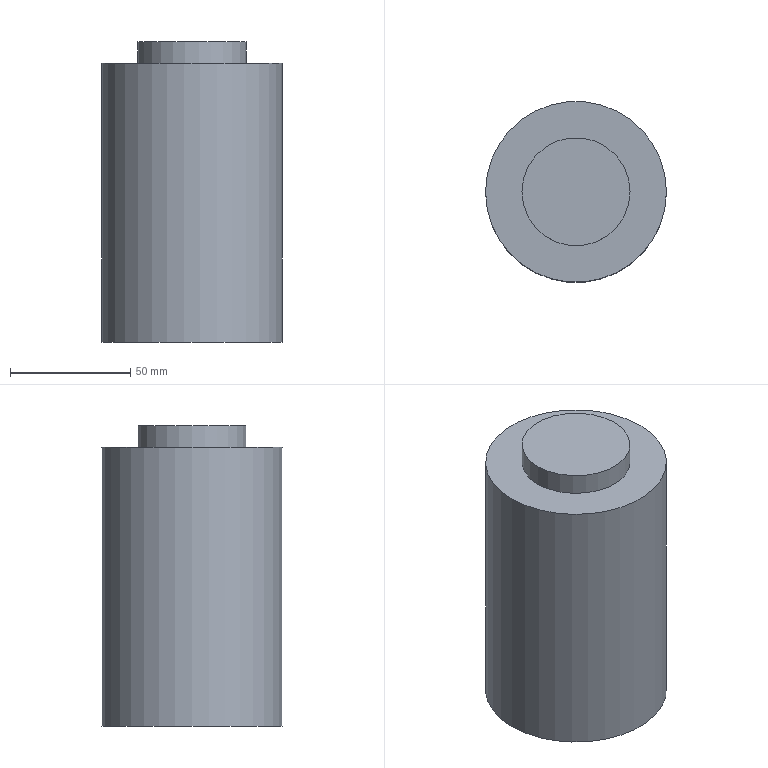Part | NX | features solid 2 | 1 solid | 5 faces | box 75.2 x 75.2 x 125 mm | volume 529523 mm3 | plane 3 | cylinder 2 | commonest cylinder face diameters 45 x1 75.2 x1
STEP:
#1=CARTESIAN_POINT('',(-1167.4,1050.,86.));
#2=VERTEX_POINT('',#1);
#3=CARTESIAN_POINT('',(-1205.,1050.,86.));
#4=DIRECTION('',(0.,0.,1.));
#5=DIRECTION('',(1.,0.,0.));
#6=AXIS2_PLACEMENT_3D('',#3,#4,#5);
#7=CIRCLE('',#6,37.6);
#8=EDGE_CURVE('',#2,#2,#7,.F.);
#9=ORIENTED_EDGE('',*,*,#8,.F.);
#10=EDGE_LOOP('',(#9));
#11=FACE_BOUND('',#10,.T.);
#12=CARTESIAN_POINT('',(-1182.5,1050.,86.));
#13=VERTEX_POINT('',#12);
#14=CARTESIAN_POINT('',(-1205.,1050.,86.));
#15=DIRECTION('',(0.,0.,1.));
#16=DIRECTION('',(1.,0.,0.));
#17=AXIS2_PLACEMENT_3D('',#14,#15,#16);
#18=CIRCLE('',#17,22.5);
#19=EDGE_CURVE('',#13,#13,#18,.F.);
#20=ORIENTED_EDGE('',*,*,#19,.T.);
#21=EDGE_LOOP('',(#20));
#22=FACE_BOUND('',#21,.T.);
#23=CARTESIAN_POINT('',(-1205.,1050.,86.));
#24=DIRECTION('',(0.,0.,1.));
#25=DIRECTION('',(1.,0.,0.));
#26=AXIS2_PLACEMENT_3D('',#23,#24,#25);
#27=PLANE('',#26);
#28=ADVANCED_FACE('',(#11,#22),#27,.T.);
#29=CARTESIAN_POINT('',(-1167.4,1050.,-30.));
#30=VERTEX_POINT('',#29);
#31=CARTESIAN_POINT('',(-1205.,1050.,-30.));
#32=DIRECTION('',(0.,0.,1.));
#33=DIRECTION('',(1.,0.,0.));
#34=AXIS2_PLACEMENT_3D('',#31,#32,#33);
#35=CIRCLE('',#34,37.6);
#36=EDGE_CURVE('',#30,#30,#35,.F.);
#37=ORIENTED_EDGE('',*,*,#36,.F.);
#38=EDGE_LOOP('',(#37));
#39=FACE_BOUND('',#38,.T.);
#40=ORIENTED_EDGE('',*,*,#8,.T.);
#41=EDGE_LOOP('',(#40));
#42=FACE_BOUND('',#41,.T.);
#43=CARTESIAN_POINT('',(-1205.,1050.,-30.));
#44=DIRECTION('',(0.,0.,1.));
#45=DIRECTION('',(1.,0.,0.));
#46=AXIS2_PLACEMENT_3D('',#43,#44,#45);
#47=CYLINDRICAL_SURFACE('',#46,37.6);
#48=ADVANCED_FACE('',(#39,#42),#47,.T.);
#49=ORIENTED_EDGE('',*,*,#36,.T.);
#50=EDGE_LOOP('',(#49));
#51=FACE_BOUND('',#50,.T.);
#52=CARTESIAN_POINT('',(-1205.,1050.,-30.));
#53=DIRECTION('',(0.,0.,1.));
#54=DIRECTION('',(1.,0.,0.));
#55=AXIS2_PLACEMENT_3D('',#52,#53,#54);
#56=PLANE('',#55);
#57=ADVANCED_FACE('',(#51),#56,.F.);
#58=CARTESIAN_POINT('',(-1182.5,1050.,95.));
#59=VERTEX_POINT('',#58);
#60=CARTESIAN_POINT('',(-1205.,1050.,95.));
#61=DIRECTION('',(0.,0.,1.));
#62=DIRECTION('',(1.,0.,0.));
#63=AXIS2_PLACEMENT_3D('',#60,#61,#62);
#64=CIRCLE('',#63,22.5);
#65=EDGE_CURVE('',#59,#59,#64,.F.);
#66=ORIENTED_EDGE('',*,*,#65,.T.);
#67=EDGE_LOOP('',(#66));
#68=FACE_BOUND('',#67,.T.);
#69=ORIENTED_EDGE('',*,*,#19,.F.);
#70=EDGE_LOOP('',(#69));
#71=FACE_BOUND('',#70,.T.);
#72=CARTESIAN_POINT('',(-1205.,1050.,164.));
#73=DIRECTION('',(0.,0.,-1.));
#74=DIRECTION('',(-1.,0.,0.));
#75=AXIS2_PLACEMENT_3D('',#72,#73,#74);
#76=CYLINDRICAL_SURFACE('',#75,22.5);
#77=ADVANCED_FACE('',(#68,#71),#76,.T.);
#78=ORIENTED_EDGE('',*,*,#65,.F.);
#79=EDGE_LOOP('',(#78));
#80=FACE_BOUND('',#79,.T.);
#81=CARTESIAN_POINT('',(-1205.,1050.,95.));
#82=DIRECTION('',(0.,0.,1.));
#83=DIRECTION('',(1.,0.,0.));
#84=AXIS2_PLACEMENT_3D('',#81,#82,#83);
#85=PLANE('',#84);
#86=ADVANCED_FACE('',(#80),#85,.T.);
#87=CLOSED_SHELL('',(#28,#48,#57,#77,#86));
#88=MANIFOLD_SOLID_BREP('',#87);
#89=(LENGTH_UNIT()NAMED_UNIT(*)SI_UNIT(.MILLI.,.METRE.));
#90=UNCERTAINTY_MEASURE_WITH_UNIT(LENGTH_MEASURE(0.00001),#89,'','');
#91=(NAMED_UNIT(*)PLANE_ANGLE_UNIT()SI_UNIT($,.RADIAN.));
#92=(NAMED_UNIT(*)SI_UNIT($,.STERADIAN.)SOLID_ANGLE_UNIT());
#93=(GEOMETRIC_REPRESENTATION_CONTEXT(3)GLOBAL_UNCERTAINTY_ASSIGNED_CONTEXT((#90))GLOBAL_UNIT_ASSIGNED_CONTEXT((#89,#91,#92))REPRESENTATION_CONTEXT('',''));
#94=ADVANCED_BREP_SHAPE_REPRESENTATION('',(#88),#93);